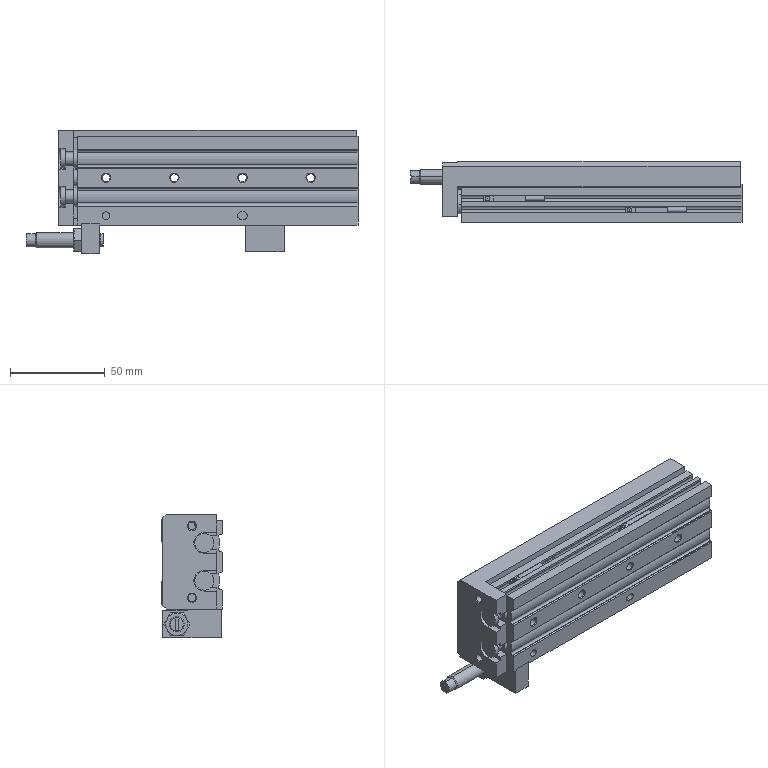Part | SolidWorks | features AEMSimFeature 1 | 8 solids | 528 faces | box 175.3 x 32 x 65 mm | volume 205284 mm3 | plane 268 | cylinder 186 | cone 72 | torus 2 | commonest cylinder face diameters 3.242 x32 4 x18 4.2 x12 7.5 x10 4.134 x8 6 x8